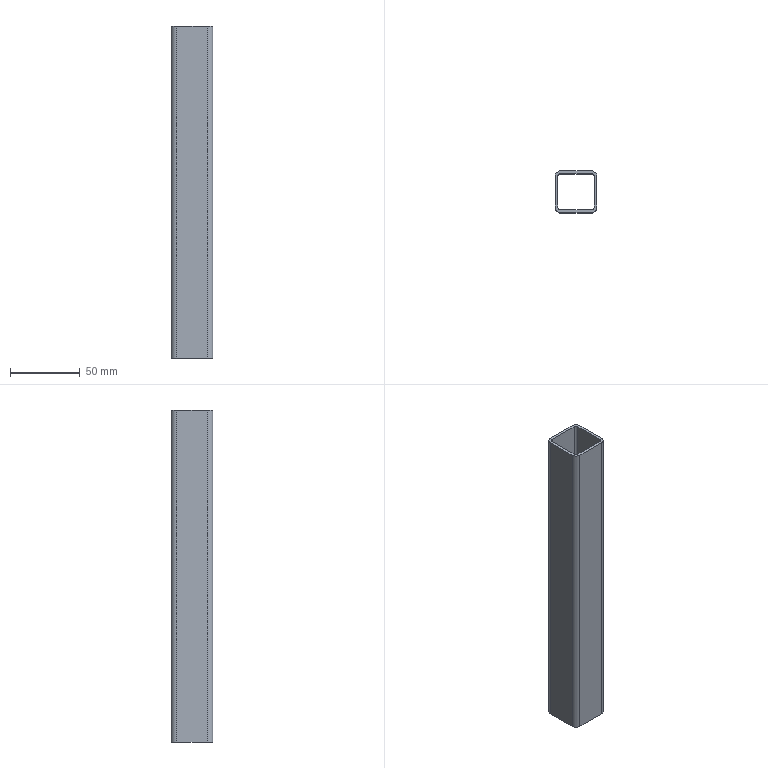Part | SolidWorks | features BaseBody 1 | 1 solid | 18 faces | box 30 x 30 x 238.5 mm | volume 50967 mm3 | plane 10 | cylinder 8 | commonest cylinder face diameters 4 x4 8 x4
STEP:
#1=CARTESIAN_POINT('',(-238.,-776.,31.5));
#2=VERTEX_POINT('',#1);
#3=CARTESIAN_POINT('',(-238.,-776.,270.));
#4=VERTEX_POINT('',#3);
#5=CARTESIAN_POINT('',(-238.,-776.,1.5));
#6=DIRECTION('',(0.,0.,1.));
#7=VECTOR('',#6,1000.);
#8=LINE('',#5,#7);
#9=EDGE_CURVE('',#2,#4,#8,.T.);
#10=ORIENTED_EDGE('',*,*,#9,.F.);
#11=CARTESIAN_POINT('',(-238.,-754.,31.5));
#12=VERTEX_POINT('',#11);
#13=CARTESIAN_POINT('',(-238.,-754.,31.5));
#14=DIRECTION('',(0.,1.,0.));
#15=VECTOR('',#14,1000.);
#16=LINE('',#13,#15);
#17=EDGE_CURVE('',#2,#12,#16,.T.);
#18=ORIENTED_EDGE('',*,*,#17,.T.);
#19=CARTESIAN_POINT('',(-238.,-754.,270.));
#20=VERTEX_POINT('',#19);
#21=CARTESIAN_POINT('',(-238.,-754.,1.5));
#22=DIRECTION('',(0.,0.,1.));
#23=VECTOR('',#22,1000.);
#24=LINE('',#21,#23);
#25=EDGE_CURVE('',#12,#20,#24,.T.);
#26=ORIENTED_EDGE('',*,*,#25,.T.);
#27=CARTESIAN_POINT('',(-238.,-754.,270.));
#28=DIRECTION('',(0.,-1.,0.));
#29=VECTOR('',#28,1000.);
#30=LINE('',#27,#29);
#31=EDGE_CURVE('',#20,#4,#30,.T.);
#32=ORIENTED_EDGE('',*,*,#31,.T.);
#33=EDGE_LOOP('',(#10,#18,#26,#32));
#34=FACE_OUTER_BOUND('',#33,.T.);
#35=CARTESIAN_POINT('',(-238.,-754.,1.5));
#36=DIRECTION('',(1.,0.,0.));
#37=DIRECTION('',(0.,0.,-1.));
#38=AXIS2_PLACEMENT_3D('',#35,#36,#37);
#39=PLANE('',#38);
#40=ADVANCED_FACE('',(#34),#39,.T.);
#41=ORIENTED_EDGE('',*,*,#25,.F.);
#42=CARTESIAN_POINT('',(-236.,-752.,31.5));
#43=VERTEX_POINT('',#42);
#44=CARTESIAN_POINT('',(-236.,-754.,31.5));
#45=DIRECTION('',(0.,0.,-1.));
#46=DIRECTION('',(-1.,0.,0.));
#47=AXIS2_PLACEMENT_3D('',#44,#45,#46);
#48=CIRCLE('',#47,2.);
#49=EDGE_CURVE('',#12,#43,#48,.T.);
#50=ORIENTED_EDGE('',*,*,#49,.T.);
#51=CARTESIAN_POINT('',(-236.,-752.,270.));
#52=VERTEX_POINT('',#51);
#53=CARTESIAN_POINT('',(-236.,-752.,1.5));
#54=DIRECTION('',(0.,0.,1.));
#55=VECTOR('',#54,1000.);
#56=LINE('',#53,#55);
#57=EDGE_CURVE('',#43,#52,#56,.T.);
#58=ORIENTED_EDGE('',*,*,#57,.T.);
#59=CARTESIAN_POINT('',(-236.,-754.,270.));
#60=DIRECTION('',(0.,0.,1.));
#61=DIRECTION('',(1.,0.,0.));
#62=AXIS2_PLACEMENT_3D('',#59,#60,#61);
#63=CIRCLE('',#62,2.);
#64=EDGE_CURVE('',#52,#20,#63,.T.);
#65=ORIENTED_EDGE('',*,*,#64,.T.);
#66=EDGE_LOOP('',(#41,#50,#58,#65));
#67=FACE_OUTER_BOUND('',#66,.T.);
#68=CARTESIAN_POINT('',(-236.,-754.,1.5));
#69=DIRECTION('',(0.,0.,1.));
#70=DIRECTION('',(1.,0.,0.));
#71=AXIS2_PLACEMENT_3D('',#68,#69,#70);
#72=CYLINDRICAL_SURFACE('',#71,2.);
#73=ADVANCED_FACE('',(#67),#72,.F.);
#74=ORIENTED_EDGE('',*,*,#57,.F.);
#75=CARTESIAN_POINT('',(-214.,-752.,31.5));
#76=VERTEX_POINT('',#75);
#77=CARTESIAN_POINT('',(-236.,-752.,31.5));
#78=DIRECTION('',(1.,0.,0.));
#79=VECTOR('',#78,1000.);
#80=LINE('',#77,#79);
#81=EDGE_CURVE('',#43,#76,#80,.T.);
#82=ORIENTED_EDGE('',*,*,#81,.T.);
#83=CARTESIAN_POINT('',(-214.,-752.,270.));
#84=VERTEX_POINT('',#83);
#85=CARTESIAN_POINT('',(-214.,-752.,1.5));
#86=DIRECTION('',(0.,0.,1.));
#87=VECTOR('',#86,1000.);
#88=LINE('',#85,#87);
#89=EDGE_CURVE('',#76,#84,#88,.T.);
#90=ORIENTED_EDGE('',*,*,#89,.T.);
#91=CARTESIAN_POINT('',(-236.,-752.,270.));
#92=DIRECTION('',(-1.,0.,0.));
#93=VECTOR('',#92,1000.);
#94=LINE('',#91,#93);
#95=EDGE_CURVE('',#84,#52,#94,.T.);
#96=ORIENTED_EDGE('',*,*,#95,.T.);
#97=EDGE_LOOP('',(#74,#82,#90,#96));
#98=FACE_OUTER_BOUND('',#97,.T.);
#99=CARTESIAN_POINT('',(-236.,-752.,1.5));
#100=DIRECTION('',(0.,-1.,0.));
#101=DIRECTION('',(0.,0.,-1.));
#102=AXIS2_PLACEMENT_3D('',#99,#100,#101);
#103=PLANE('',#102);
#104=ADVANCED_FACE('',(#98),#103,.T.);
#105=ORIENTED_EDGE('',*,*,#89,.F.);
#106=CARTESIAN_POINT('',(-212.,-754.,31.5));
#107=VERTEX_POINT('',#106);
#108=CARTESIAN_POINT('',(-214.,-754.,31.5));
#109=DIRECTION('',(0.,0.,-1.));
#110=DIRECTION('',(-1.,0.,0.));
#111=AXIS2_PLACEMENT_3D('',#108,#109,#110);
#112=CIRCLE('',#111,2.);
#113=EDGE_CURVE('',#76,#107,#112,.T.);
#114=ORIENTED_EDGE('',*,*,#113,.T.);
#115=CARTESIAN_POINT('',(-212.,-754.,270.));
#116=VERTEX_POINT('',#115);
#117=CARTESIAN_POINT('',(-212.,-754.,1.5));
#118=DIRECTION('',(0.,0.,1.));
#119=VECTOR('',#118,1000.);
#120=LINE('',#117,#119);
#121=EDGE_CURVE('',#107,#116,#120,.T.);
#122=ORIENTED_EDGE('',*,*,#121,.T.);
#123=CARTESIAN_POINT('',(-214.,-754.,270.));
#124=DIRECTION('',(0.,0.,1.));
#125=DIRECTION('',(1.,0.,0.));
#126=AXIS2_PLACEMENT_3D('',#123,#124,#125);
#127=CIRCLE('',#126,2.);
#128=EDGE_CURVE('',#116,#84,#127,.T.);
#129=ORIENTED_EDGE('',*,*,#128,.T.);
#130=EDGE_LOOP('',(#105,#114,#122,#129));
#131=FACE_OUTER_BOUND('',#130,.T.);
#132=CARTESIAN_POINT('',(-214.,-754.,1.5));
#133=DIRECTION('',(0.,0.,1.));
#134=DIRECTION('',(1.,0.,0.));
#135=AXIS2_PLACEMENT_3D('',#132,#133,#134);
#136=CYLINDRICAL_SURFACE('',#135,2.);
#137=ADVANCED_FACE('',(#131),#136,.F.);
#138=ORIENTED_EDGE('',*,*,#121,.F.);
#139=CARTESIAN_POINT('',(-212.,-776.,31.5));
#140=VERTEX_POINT('',#139);
#141=CARTESIAN_POINT('',(-212.,-776.,31.5));
#142=DIRECTION('',(0.,-1.,0.));
#143=VECTOR('',#142,1000.);
#144=LINE('',#141,#143);
#145=EDGE_CURVE('',#107,#140,#144,.T.);
#146=ORIENTED_EDGE('',*,*,#145,.T.);
#147=CARTESIAN_POINT('',(-212.,-776.,270.));
#148=VERTEX_POINT('',#147);
#149=CARTESIAN_POINT('',(-212.,-776.,1.5));
#150=DIRECTION('',(0.,0.,1.));
#151=VECTOR('',#150,1000.);
#152=LINE('',#149,#151);
#153=EDGE_CURVE('',#140,#148,#152,.T.);
#154=ORIENTED_EDGE('',*,*,#153,.T.);
#155=CARTESIAN_POINT('',(-212.,-776.,270.));
#156=DIRECTION('',(0.,1.,0.));
#157=VECTOR('',#156,1000.);
#158=LINE('',#155,#157);
#159=EDGE_CURVE('',#148,#116,#158,.T.);
#160=ORIENTED_EDGE('',*,*,#159,.T.);
#161=EDGE_LOOP('',(#138,#146,#154,#160));
#162=FACE_OUTER_BOUND('',#161,.T.);
#163=CARTESIAN_POINT('',(-212.,-776.,1.5));
#164=DIRECTION('',(-1.,0.,0.));
#165=DIRECTION('',(0.,0.,1.));
#166=AXIS2_PLACEMENT_3D('',#163,#164,#165);
#167=PLANE('',#166);
#168=ADVANCED_FACE('',(#162),#167,.T.);
#169=ORIENTED_EDGE('',*,*,#153,.F.);
#170=CARTESIAN_POINT('',(-214.,-778.,31.5));
#171=VERTEX_POINT('',#170);
#172=CARTESIAN_POINT('',(-214.,-776.,31.5));
#173=DIRECTION('',(0.,0.,-1.));
#174=DIRECTION('',(-1.,0.,0.));
#175=AXIS2_PLACEMENT_3D('',#172,#173,#174);
#176=CIRCLE('',#175,2.);
#177=EDGE_CURVE('',#140,#171,#176,.T.);
#178=ORIENTED_EDGE('',*,*,#177,.T.);
#179=CARTESIAN_POINT('',(-214.,-778.,270.));
#180=VERTEX_POINT('',#179);
#181=CARTESIAN_POINT('',(-214.,-778.,1.5));
#182=DIRECTION('',(0.,0.,1.));
#183=VECTOR('',#182,1000.);
#184=LINE('',#181,#183);
#185=EDGE_CURVE('',#171,#180,#184,.T.);
#186=ORIENTED_EDGE('',*,*,#185,.T.);
#187=CARTESIAN_POINT('',(-214.,-776.,270.));
#188=DIRECTION('',(0.,0.,1.));
#189=DIRECTION('',(1.,0.,0.));
#190=AXIS2_PLACEMENT_3D('',#187,#188,#189);
#191=CIRCLE('',#190,2.);
#192=EDGE_CURVE('',#180,#148,#191,.T.);
#193=ORIENTED_EDGE('',*,*,#192,.T.);
#194=EDGE_LOOP('',(#169,#178,#186,#193));
#195=FACE_OUTER_BOUND('',#194,.T.);
#196=CARTESIAN_POINT('',(-214.,-776.,1.5));
#197=DIRECTION('',(0.,0.,1.));
#198=DIRECTION('',(1.,0.,0.));
#199=AXIS2_PLACEMENT_3D('',#196,#197,#198);
#200=CYLINDRICAL_SURFACE('',#199,2.);
#201=ADVANCED_FACE('',(#195),#200,.F.);
#202=ORIENTED_EDGE('',*,*,#185,.F.);
#203=CARTESIAN_POINT('',(-236.,-778.,31.5));
#204=VERTEX_POINT('',#203);
#205=CARTESIAN_POINT('',(-214.,-778.,31.5));
#206=DIRECTION('',(-1.,0.,0.));
#207=VECTOR('',#206,1000.);
#208=LINE('',#205,#207);
#209=EDGE_CURVE('',#171,#204,#208,.T.);
#210=ORIENTED_EDGE('',*,*,#209,.T.);
#211=CARTESIAN_POINT('',(-236.,-778.,270.));
#212=VERTEX_POINT('',#211);
#213=CARTESIAN_POINT('',(-236.,-778.,1.5));
#214=DIRECTION('',(0.,0.,1.));
#215=VECTOR('',#214,1000.);
#216=LINE('',#213,#215);
#217=EDGE_CURVE('',#204,#212,#216,.T.);
#218=ORIENTED_EDGE('',*,*,#217,.T.);
#219=CARTESIAN_POINT('',(-214.,-778.,270.));
#220=DIRECTION('',(1.,0.,0.));
#221=VECTOR('',#220,1000.);
#222=LINE('',#219,#221);
#223=EDGE_CURVE('',#212,#180,#222,.T.);
#224=ORIENTED_EDGE('',*,*,#223,.T.);
#225=EDGE_LOOP('',(#202,#210,#218,#224));
#226=FACE_OUTER_BOUND('',#225,.T.);
#227=CARTESIAN_POINT('',(-214.,-778.,1.5));
#228=DIRECTION('',(0.,1.,0.));
#229=DIRECTION('',(0.,0.,1.));
#230=AXIS2_PLACEMENT_3D('',#227,#228,#229);
#231=PLANE('',#230);
#232=ADVANCED_FACE('',(#226),#231,.T.);
#233=ORIENTED_EDGE('',*,*,#217,.F.);
#234=CARTESIAN_POINT('',(-236.,-776.,31.5));
#235=DIRECTION('',(0.,0.,-1.));
#236=DIRECTION('',(-1.,0.,0.));
#237=AXIS2_PLACEMENT_3D('',#234,#235,#236);
#238=CIRCLE('',#237,2.);
#239=EDGE_CURVE('',#204,#2,#238,.T.);
#240=ORIENTED_EDGE('',*,*,#239,.T.);
#241=ORIENTED_EDGE('',*,*,#9,.T.);
#242=CARTESIAN_POINT('',(-236.,-776.,270.));
#243=DIRECTION('',(0.,0.,1.));
#244=DIRECTION('',(1.,0.,0.));
#245=AXIS2_PLACEMENT_3D('',#242,#243,#244);
#246=CIRCLE('',#245,2.);
#247=EDGE_CURVE('',#4,#212,#246,.T.);
#248=ORIENTED_EDGE('',*,*,#247,.T.);
#249=EDGE_LOOP('',(#233,#240,#241,#248));
#250=FACE_OUTER_BOUND('',#249,.T.);
#251=CARTESIAN_POINT('',(-236.,-776.,1.5));
#252=DIRECTION('',(0.,0.,1.));
#253=DIRECTION('',(1.,0.,0.));
#254=AXIS2_PLACEMENT_3D('',#251,#252,#253);
#255=CYLINDRICAL_SURFACE('',#254,2.);
#256=ADVANCED_FACE('',(#250),#255,.F.);
#257=CARTESIAN_POINT('',(-210.,-754.,31.5));
#258=VERTEX_POINT('',#257);
#259=CARTESIAN_POINT('',(-210.,-776.,31.5));
#260=VERTEX_POINT('',#259);
#261=CARTESIAN_POINT('',(-210.,-776.,31.5));
#262=DIRECTION('',(0.,-1.,0.));
#263=VECTOR('',#262,1000.);
#264=LINE('',#261,#263);
#265=EDGE_CURVE('',#258,#260,#264,.T.);
#266=ORIENTED_EDGE('',*,*,#265,.F.);
#267=CARTESIAN_POINT('',(-210.,-754.,270.));
#268=VERTEX_POINT('',#267);
#269=CARTESIAN_POINT('',(-210.,-754.,1.5));
#270=DIRECTION('',(0.,0.,1.));
#271=VECTOR('',#270,1000.);
#272=LINE('',#269,#271);
#273=EDGE_CURVE('',#258,#268,#272,.T.);
#274=ORIENTED_EDGE('',*,*,#273,.T.);
#275=CARTESIAN_POINT('',(-210.,-776.,270.));
#276=VERTEX_POINT('',#275);
#277=CARTESIAN_POINT('',(-210.,-776.,270.));
#278=DIRECTION('',(0.,1.,0.));
#279=VECTOR('',#278,1000.);
#280=LINE('',#277,#279);
#281=EDGE_CURVE('',#276,#268,#280,.T.);
#282=ORIENTED_EDGE('',*,*,#281,.F.);
#283=CARTESIAN_POINT('',(-210.,-776.,1.5));
#284=DIRECTION('',(0.,0.,1.));
#285=VECTOR('',#284,1000.);
#286=LINE('',#283,#285);
#287=EDGE_CURVE('',#260,#276,#286,.T.);
#288=ORIENTED_EDGE('',*,*,#287,.F.);
#289=EDGE_LOOP('',(#266,#274,#282,#288));
#290=FACE_OUTER_BOUND('',#289,.T.);
#291=CARTESIAN_POINT('',(-210.,-776.,1.5));
#292=DIRECTION('',(-1.,0.,0.));
#293=DIRECTION('',(0.,0.,1.));
#294=AXIS2_PLACEMENT_3D('',#291,#292,#293);
#295=PLANE('',#294);
#296=ADVANCED_FACE('',(#290),#295,.F.);
#297=CARTESIAN_POINT('',(-214.,-750.,31.5));
#298=VERTEX_POINT('',#297);
#299=CARTESIAN_POINT('',(-214.,-754.,31.5));
#300=DIRECTION('',(0.,0.,-1.));
#301=DIRECTION('',(-1.,0.,0.));
#302=AXIS2_PLACEMENT_3D('',#299,#300,#301);
#303=CIRCLE('',#302,4.);
#304=EDGE_CURVE('',#298,#258,#303,.T.);
#305=ORIENTED_EDGE('',*,*,#304,.F.);
#306=CARTESIAN_POINT('',(-214.,-750.,270.));
#307=VERTEX_POINT('',#306);
#308=CARTESIAN_POINT('',(-214.,-750.,1.5));
#309=DIRECTION('',(0.,0.,1.));
#310=VECTOR('',#309,1000.);
#311=LINE('',#308,#310);
#312=EDGE_CURVE('',#298,#307,#311,.T.);
#313=ORIENTED_EDGE('',*,*,#312,.T.);
#314=CARTESIAN_POINT('',(-214.,-754.,270.));
#315=DIRECTION('',(0.,0.,1.));
#316=DIRECTION('',(1.,0.,0.));
#317=AXIS2_PLACEMENT_3D('',#314,#315,#316);
#318=CIRCLE('',#317,4.);
#319=EDGE_CURVE('',#268,#307,#318,.T.);
#320=ORIENTED_EDGE('',*,*,#319,.F.);
#321=ORIENTED_EDGE('',*,*,#273,.F.);
#322=EDGE_LOOP('',(#305,#313,#320,#321));
#323=FACE_OUTER_BOUND('',#322,.T.);
#324=CARTESIAN_POINT('',(-214.,-754.,1.5));
#325=DIRECTION('',(0.,0.,1.));
#326=DIRECTION('',(1.,0.,0.));
#327=AXIS2_PLACEMENT_3D('',#324,#325,#326);
#328=CYLINDRICAL_SURFACE('',#327,4.);
#329=ADVANCED_FACE('',(#323),#328,.T.);
#330=CARTESIAN_POINT('',(-236.,-750.,31.5));
#331=VERTEX_POINT('',#330);
#332=CARTESIAN_POINT('',(373.,-750.,31.5));
#333=DIRECTION('',(-1.,0.,0.));
#334=VECTOR('',#333,1000.);
#335=LINE('',#332,#334);
#336=EDGE_CURVE('',#298,#331,#335,.T.);
#337=ORIENTED_EDGE('',*,*,#336,.T.);
#338=CARTESIAN_POINT('',(-236.,-750.,270.));
#339=VERTEX_POINT('',#338);
#340=CARTESIAN_POINT('',(-236.,-750.,1.5));
#341=DIRECTION('',(0.,0.,1.));
#342=VECTOR('',#341,1000.);
#343=LINE('',#340,#342);
#344=EDGE_CURVE('',#331,#339,#343,.T.);
#345=ORIENTED_EDGE('',*,*,#344,.T.);
#346=CARTESIAN_POINT('',(375.,-750.,270.));
#347=DIRECTION('',(-1.,0.,0.));
#348=VECTOR('',#347,1000.);
#349=LINE('',#346,#348);
#350=EDGE_CURVE('',#307,#339,#349,.T.);
#351=ORIENTED_EDGE('',*,*,#350,.F.);
#352=ORIENTED_EDGE('',*,*,#312,.F.);
#353=EDGE_LOOP('',(#337,#345,#351,#352));
#354=FACE_OUTER_BOUND('',#353,.T.);
#355=CARTESIAN_POINT('',(-236.,-750.,1.5));
#356=DIRECTION('',(0.,-1.,0.));
#357=DIRECTION('',(0.,0.,-1.));
#358=AXIS2_PLACEMENT_3D('',#355,#356,#357);
#359=PLANE('',#358);
#360=ADVANCED_FACE('',(#354),#359,.F.);
#361=CARTESIAN_POINT('',(-240.,-754.,31.5));
#362=VERTEX_POINT('',#361);
#363=CARTESIAN_POINT('',(-236.,-754.,31.5));
#364=DIRECTION('',(0.,0.,-1.));
#365=DIRECTION('',(-1.,0.,0.));
#366=AXIS2_PLACEMENT_3D('',#363,#364,#365);
#367=CIRCLE('',#366,4.);
#368=EDGE_CURVE('',#362,#331,#367,.T.);
#369=ORIENTED_EDGE('',*,*,#368,.F.);
#370=CARTESIAN_POINT('',(-240.,-754.,270.));
#371=VERTEX_POINT('',#370);
#372=CARTESIAN_POINT('',(-240.,-754.,1.5));
#373=DIRECTION('',(0.,0.,1.));
#374=VECTOR('',#373,1000.);
#375=LINE('',#372,#374);
#376=EDGE_CURVE('',#362,#371,#375,.T.);
#377=ORIENTED_EDGE('',*,*,#376,.T.);
#378=CARTESIAN_POINT('',(-236.,-754.,270.));
#379=DIRECTION('',(0.,0.,1.));
#380=DIRECTION('',(1.,0.,0.));
#381=AXIS2_PLACEMENT_3D('',#378,#379,#380);
#382=CIRCLE('',#381,4.);
#383=EDGE_CURVE('',#339,#371,#382,.T.);
#384=ORIENTED_EDGE('',*,*,#383,.F.);
#385=ORIENTED_EDGE('',*,*,#344,.F.);
#386=EDGE_LOOP('',(#369,#377,#384,#385));
#387=FACE_OUTER_BOUND('',#386,.T.);
#388=CARTESIAN_POINT('',(-236.,-754.,1.5));
#389=DIRECTION('',(0.,0.,1.));
#390=DIRECTION('',(1.,0.,0.));
#391=AXIS2_PLACEMENT_3D('',#388,#389,#390);
#392=CYLINDRICAL_SURFACE('',#391,4.);
#393=ADVANCED_FACE('',(#387),#392,.T.);
#394=CARTESIAN_POINT('',(-240.,-776.,31.5));
#395=VERTEX_POINT('',#394);
#396=CARTESIAN_POINT('',(-240.,-754.,31.5));
#397=DIRECTION('',(0.,1.,0.));
#398=VECTOR('',#397,1000.);
#399=LINE('',#396,#398);
#400=EDGE_CURVE('',#395,#362,#399,.T.);
#401=ORIENTED_EDGE('',*,*,#400,.F.);
#402=CARTESIAN_POINT('',(-240.,-776.,270.));
#403=VERTEX_POINT('',#402);
#404=CARTESIAN_POINT('',(-240.,-776.,1.5));
#405=DIRECTION('',(0.,0.,1.));
#406=VECTOR('',#405,1000.);
#407=LINE('',#404,#406);
#408=EDGE_CURVE('',#395,#403,#407,.T.);
#409=ORIENTED_EDGE('',*,*,#408,.T.);
#410=CARTESIAN_POINT('',(-240.,-754.,270.));
#411=DIRECTION('',(0.,-1.,0.));
#412=VECTOR('',#411,1000.);
#413=LINE('',#410,#412);
#414=EDGE_CURVE('',#371,#403,#413,.T.);
#415=ORIENTED_EDGE('',*,*,#414,.F.);
#416=ORIENTED_EDGE('',*,*,#376,.F.);
#417=EDGE_LOOP('',(#401,#409,#415,#416));
#418=FACE_OUTER_BOUND('',#417,.T.);
#419=CARTESIAN_POINT('',(-240.,-754.,1.5));
#420=DIRECTION('',(1.,0.,0.));
#421=DIRECTION('',(0.,0.,-1.));
#422=AXIS2_PLACEMENT_3D('',#419,#420,#421);
#423=PLANE('',#422);
#424=ADVANCED_FACE('',(#418),#423,.F.);
#425=CARTESIAN_POINT('',(-236.,-780.,31.5));
#426=VERTEX_POINT('',#425);
#427=CARTESIAN_POINT('',(-236.,-776.,31.5));
#428=DIRECTION('',(0.,0.,-1.));
#429=DIRECTION('',(-1.,0.,0.));
#430=AXIS2_PLACEMENT_3D('',#427,#428,#429);
#431=CIRCLE('',#430,4.);
#432=EDGE_CURVE('',#426,#395,#431,.T.);
#433=ORIENTED_EDGE('',*,*,#432,.F.);
#434=CARTESIAN_POINT('',(-236.,-780.,270.));
#435=VERTEX_POINT('',#434);
#436=CARTESIAN_POINT('',(-236.,-780.,1.5));
#437=DIRECTION('',(0.,0.,1.));
#438=VECTOR('',#437,1000.);
#439=LINE('',#436,#438);
#440=EDGE_CURVE('',#426,#435,#439,.T.);
#441=ORIENTED_EDGE('',*,*,#440,.T.);
#442=CARTESIAN_POINT('',(-236.,-776.,270.));
#443=DIRECTION('',(0.,0.,1.));
#444=DIRECTION('',(1.,0.,0.));
#445=AXIS2_PLACEMENT_3D('',#442,#443,#444);
#446=CIRCLE('',#445,4.);
#447=EDGE_CURVE('',#403,#435,#446,.T.);
#448=ORIENTED_EDGE('',*,*,#447,.F.);
#449=ORIENTED_EDGE('',*,*,#408,.F.);
#450=EDGE_LOOP('',(#433,#441,#448,#449));
#451=FACE_OUTER_BOUND('',#450,.T.);
#452=CARTESIAN_POINT('',(-236.,-776.,1.5));
#453=DIRECTION('',(0.,0.,1.));
#454=DIRECTION('',(1.,0.,0.));
#455=AXIS2_PLACEMENT_3D('',#452,#453,#454);
#456=CYLINDRICAL_SURFACE('',#455,4.);
#457=ADVANCED_FACE('',(#451),#456,.T.);
#458=CARTESIAN_POINT('',(-214.,-780.,31.5));
#459=VERTEX_POINT('',#458);
#460=CARTESIAN_POINT('',(373.,-780.,31.5));
#461=DIRECTION('',(-1.,0.,0.));
#462=VECTOR('',#461,1000.);
#463=LINE('',#460,#462);
#464=EDGE_CURVE('',#459,#426,#463,.T.);
#465=ORIENTED_EDGE('',*,*,#464,.F.);
#466=CARTESIAN_POINT('',(-214.,-780.,270.));
#467=VERTEX_POINT('',#466);
#468=CARTESIAN_POINT('',(-214.,-780.,1.5));
#469=DIRECTION('',(0.,0.,1.));
#470=VECTOR('',#469,1000.);
#471=LINE('',#468,#470);
#472=EDGE_CURVE('',#459,#467,#471,.T.);
#473=ORIENTED_EDGE('',*,*,#472,.T.);
#474=CARTESIAN_POINT('',(375.,-780.,270.));
#475=DIRECTION('',(-1.,0.,0.));
#476=VECTOR('',#475,1000.);
#477=LINE('',#474,#476);
#478=EDGE_CURVE('',#467,#435,#477,.T.);
#479=ORIENTED_EDGE('',*,*,#478,.T.);
#480=ORIENTED_EDGE('',*,*,#440,.F.);
#481=EDGE_LOOP('',(#465,#473,#479,#480));
#482=FACE_OUTER_BOUND('',#481,.T.);
#483=CARTESIAN_POINT('',(-214.,-780.,1.5));
#484=DIRECTION('',(0.,1.,0.));
#485=DIRECTION('',(0.,0.,1.));
#486=AXIS2_PLACEMENT_3D('',#483,#484,#485);
#487=PLANE('',#486);
#488=ADVANCED_FACE('',(#482),#487,.F.);
#489=CARTESIAN_POINT('',(-214.,-776.,31.5));
#490=DIRECTION('',(0.,0.,-1.));
#491=DIRECTION('',(-1.,0.,0.));
#492=AXIS2_PLACEMENT_3D('',#489,#490,#491);
#493=CIRCLE('',#492,4.);
#494=EDGE_CURVE('',#260,#459,#493,.T.);
#495=ORIENTED_EDGE('',*,*,#494,.F.);
#496=ORIENTED_EDGE('',*,*,#287,.T.);
#497=CARTESIAN_POINT('',(-214.,-776.,270.));
#498=DIRECTION('',(0.,0.,1.));
#499=DIRECTION('',(1.,0.,0.));
#500=AXIS2_PLACEMENT_3D('',#497,#498,#499);
#501=CIRCLE('',#500,4.);
#502=EDGE_CURVE('',#467,#276,#501,.T.);
#503=ORIENTED_EDGE('',*,*,#502,.F.);
#504=ORIENTED_EDGE('',*,*,#472,.F.);
#505=EDGE_LOOP('',(#495,#496,#503,#504));
#506=FACE_OUTER_BOUND('',#505,.T.);
#507=CARTESIAN_POINT('',(-214.,-776.,1.5));
#508=DIRECTION('',(0.,0.,1.));
#509=DIRECTION('',(1.,0.,0.));
#510=AXIS2_PLACEMENT_3D('',#507,#508,#509);
#511=CYLINDRICAL_SURFACE('',#510,4.);
#512=ADVANCED_FACE('',(#506),#511,.T.);
#513=ORIENTED_EDGE('',*,*,#31,.F.);
#514=ORIENTED_EDGE('',*,*,#64,.F.);
#515=ORIENTED_EDGE('',*,*,#95,.F.);
#516=ORIENTED_EDGE('',*,*,#128,.F.);
#517=ORIENTED_EDGE('',*,*,#159,.F.);
#518=ORIENTED_EDGE('',*,*,#192,.F.);
#519=ORIENTED_EDGE('',*,*,#223,.F.);
#520=ORIENTED_EDGE('',*,*,#247,.F.);
#521=EDGE_LOOP('',(#513,#514,#515,#516,#517,#518,#519,#520));
#522=FACE_BOUND('',#521,.T.);
#523=ORIENTED_EDGE('',*,*,#447,.T.);
#524=ORIENTED_EDGE('',*,*,#478,.F.);
#525=ORIENTED_EDGE('',*,*,#502,.T.);
#526=ORIENTED_EDGE('',*,*,#281,.T.);
#527=ORIENTED_EDGE('',*,*,#319,.T.);
#528=ORIENTED_EDGE('',*,*,#350,.T.);
#529=ORIENTED_EDGE('',*,*,#383,.T.);
#530=ORIENTED_EDGE('',*,*,#414,.T.);
#531=EDGE_LOOP('',(#523,#524,#525,#526,#527,#528,#529,#530));
#532=FACE_OUTER_BOUND('',#531,.T.);
#533=CARTESIAN_POINT('',(375.,-754.,270.));
#534=DIRECTION('',(0.,0.,1.));
#535=DIRECTION('',(1.,0.,0.));
#536=AXIS2_PLACEMENT_3D('',#533,#534,#535);
#537=PLANE('',#536);
#538=ADVANCED_FACE('',(#522,#532),#537,.T.);
#539=ORIENTED_EDGE('',*,*,#239,.F.);
#540=ORIENTED_EDGE('',*,*,#209,.F.);
#541=ORIENTED_EDGE('',*,*,#177,.F.);
#542=ORIENTED_EDGE('',*,*,#145,.F.);
#543=ORIENTED_EDGE('',*,*,#113,.F.);
#544=ORIENTED_EDGE('',*,*,#81,.F.);
#545=ORIENTED_EDGE('',*,*,#49,.F.);
#546=ORIENTED_EDGE('',*,*,#17,.F.);
#547=EDGE_LOOP('',(#539,#540,#541,#542,#543,#544,#545,#546));
#548=FACE_BOUND('',#547,.T.);
#549=ORIENTED_EDGE('',*,*,#368,.T.);
#550=ORIENTED_EDGE('',*,*,#336,.F.);
#551=ORIENTED_EDGE('',*,*,#304,.T.);
#552=ORIENTED_EDGE('',*,*,#265,.T.);
#553=ORIENTED_EDGE('',*,*,#494,.T.);
#554=ORIENTED_EDGE('',*,*,#464,.T.);
#555=ORIENTED_EDGE('',*,*,#432,.T.);
#556=ORIENTED_EDGE('',*,*,#400,.T.);
#557=EDGE_LOOP('',(#549,#550,#551,#552,#553,#554,#555,#556));
#558=FACE_OUTER_BOUND('',#557,.T.);
#559=CARTESIAN_POINT('',(373.,-776.,31.5));
#560=DIRECTION('',(0.,0.,-1.));
#561=DIRECTION('',(-1.,0.,0.));
#562=AXIS2_PLACEMENT_3D('',#559,#560,#561);
#563=PLANE('',#562);
#564=ADVANCED_FACE('',(#548,#558),#563,.T.);
#565=CLOSED_SHELL('',(#40,#73,#104,#137,#168,#201,#232,#256,#296,#329,#360,#393,#424,#457,#488,#512,#538,#564));
#566=MANIFOLD_SOLID_BREP('',#565);
#567=CARTESIAN_POINT('',(0.,0.,0.));
#568=DIRECTION('',(0.,0.,1.));
#569=DIRECTION('',(1.,0.,0.));
#570=AXIS2_PLACEMENT_3D('',#567,#568,#569);
#571=(LENGTH_UNIT()NAMED_UNIT(*)SI_UNIT(.MILLI.,.METRE.));
#572=UNCERTAINTY_MEASURE_WITH_UNIT(LENGTH_MEASURE(0.00001),#571,'','');
#573=(NAMED_UNIT(*)PLANE_ANGLE_UNIT()SI_UNIT($,.RADIAN.));
#574=(NAMED_UNIT(*)SI_UNIT($,.STERADIAN.)SOLID_ANGLE_UNIT());
#575=(GEOMETRIC_REPRESENTATION_CONTEXT(3)GLOBAL_UNCERTAINTY_ASSIGNED_CONTEXT((#572))GLOBAL_UNIT_ASSIGNED_CONTEXT((#571,#573,#574))REPRESENTATION_CONTEXT('',''));
#576=ADVANCED_BREP_SHAPE_REPRESENTATION('',(#566,#570),#575);